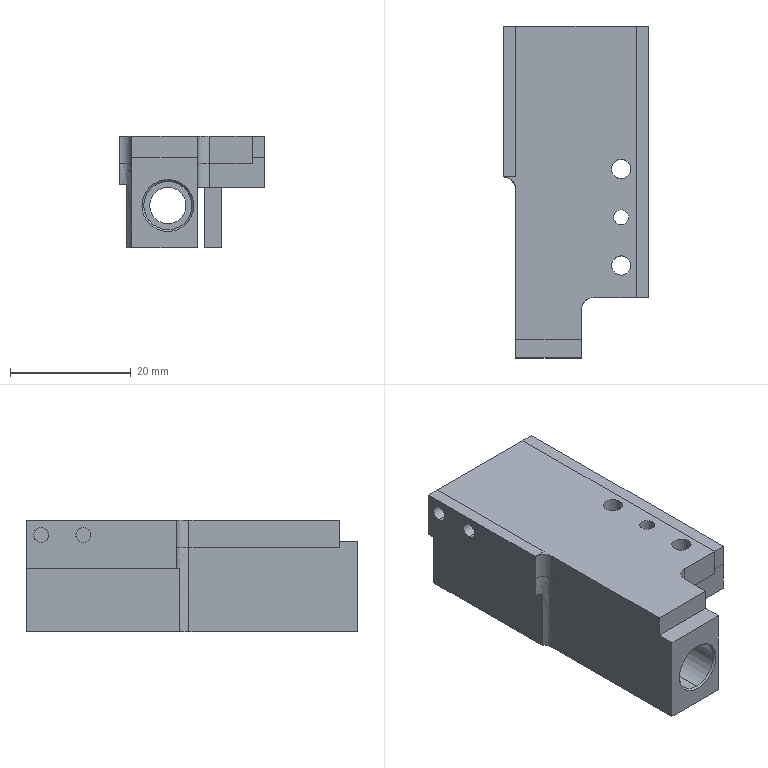Part | 3 solids | 85 faces | box 24.15 x 55 x 18.5 mm | volume 11588 mm3 | plane 48 | cylinder 27 | spline 10 | commonest cylinder face diameters 2.5 x11 3.2 x6 6.5 x4 8 x4 6 x2